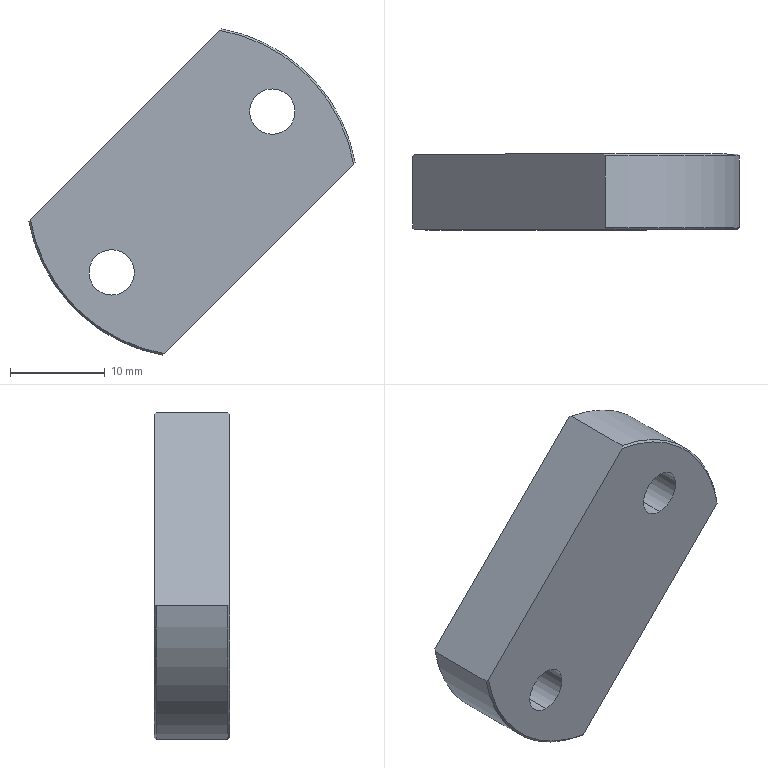Part | SolidWorks | features ICE 3, 3DProfileFeature 2, Chamfer 2, HoleWzd 2, Fillet 1, Revolution 1 | 1 solid | 20 faces | box 34.452 x 8 x 34.452 mm | volume 4691 mm3 | cylinder 10 | plane 6 | cone 4 | commonest cylinder face diameters 4.8 x4 8 x4 35 x2
STEP:
#1=CARTESIAN_POINT('',(-8.485,19.4,-12.485));
#2=VERTEX_POINT('',#1);
#3=CARTESIAN_POINT('',(-8.485,19.4,-4.485));
#4=VERTEX_POINT('',#3);
#5=CARTESIAN_POINT('',(-8.485,19.4,-8.485));
#6=DIRECTION('',(0.,1.,0.));
#7=DIRECTION('',(0.,0.,1.));
#8=AXIS2_PLACEMENT_3D('',#5,#6,#7);
#9=CIRCLE('',#8,4.);
#10=EDGE_CURVE('',#2,#4,#9,.T.);
#11=ORIENTED_EDGE('',*,*,#10,.F.);
#12=CARTESIAN_POINT('',(-8.485,24.,-12.485));
#13=VERTEX_POINT('',#12);
#14=CARTESIAN_POINT('',(-8.485,24.,-12.485));
#15=DIRECTION('',(0.,1.,0.));
#16=VECTOR('',#15,1000.);
#17=LINE('',#14,#16);
#18=EDGE_CURVE('',#2,#13,#17,.T.);
#19=ORIENTED_EDGE('',*,*,#18,.T.);
#20=CARTESIAN_POINT('',(-8.485,24.,-4.485));
#21=VERTEX_POINT('',#20);
#22=CARTESIAN_POINT('',(-8.485,24.,-8.485));
#23=DIRECTION('',(0.,1.,0.));
#24=DIRECTION('',(0.,0.,1.));
#25=AXIS2_PLACEMENT_3D('',#22,#23,#24);
#26=CIRCLE('',#25,4.);
#27=EDGE_CURVE('',#13,#21,#26,.T.);
#28=ORIENTED_EDGE('',*,*,#27,.T.);
#29=CARTESIAN_POINT('',(-8.485,24.,-4.485));
#30=DIRECTION('',(0.,1.,0.));
#31=VECTOR('',#30,1000.);
#32=LINE('',#29,#31);
#33=EDGE_CURVE('',#4,#21,#32,.T.);
#34=ORIENTED_EDGE('',*,*,#33,.F.);
#35=EDGE_LOOP('',(#11,#19,#28,#34));
#36=FACE_OUTER_BOUND('',#35,.T.);
#37=CARTESIAN_POINT('',(-8.485,24.,-8.485));
#38=DIRECTION('',(0.,1.,0.));
#39=DIRECTION('',(0.,0.,1.));
#40=AXIS2_PLACEMENT_3D('',#37,#38,#39);
#41=CYLINDRICAL_SURFACE('',#40,4.);
#42=ADVANCED_FACE('',(#36),#41,.F.);
#43=CARTESIAN_POINT('',(-8.485,16.,-10.885));
#44=VERTEX_POINT('',#43);
#45=CARTESIAN_POINT('',(-8.485,16.,-6.085));
#46=VERTEX_POINT('',#45);
#47=CARTESIAN_POINT('',(-8.485,16.,-8.485));
#48=DIRECTION('',(0.,1.,0.));
#49=DIRECTION('',(0.,0.,1.));
#50=AXIS2_PLACEMENT_3D('',#47,#48,#49);
#51=CIRCLE('',#50,2.4);
#52=EDGE_CURVE('',#44,#46,#51,.T.);
#53=ORIENTED_EDGE('',*,*,#52,.F.);
#54=CARTESIAN_POINT('',(-8.485,19.4,-10.885));
#55=VERTEX_POINT('',#54);
#56=CARTESIAN_POINT('',(-8.485,24.,-10.885));
#57=DIRECTION('',(0.,1.,0.));
#58=VECTOR('',#57,1000.);
#59=LINE('',#56,#58);
#60=EDGE_CURVE('',#44,#55,#59,.T.);
#61=ORIENTED_EDGE('',*,*,#60,.T.);
#62=CARTESIAN_POINT('',(-8.485,19.4,-6.085));
#63=VERTEX_POINT('',#62);
#64=CARTESIAN_POINT('',(-8.485,19.4,-8.485));
#65=DIRECTION('',(0.,1.,0.));
#66=DIRECTION('',(0.,0.,1.));
#67=AXIS2_PLACEMENT_3D('',#64,#65,#66);
#68=CIRCLE('',#67,2.4);
#69=EDGE_CURVE('',#55,#63,#68,.T.);
#70=ORIENTED_EDGE('',*,*,#69,.T.);
#71=CARTESIAN_POINT('',(-8.485,24.,-6.085));
#72=DIRECTION('',(0.,1.,0.));
#73=VECTOR('',#72,1000.);
#74=LINE('',#71,#73);
#75=EDGE_CURVE('',#46,#63,#74,.T.);
#76=ORIENTED_EDGE('',*,*,#75,.F.);
#77=EDGE_LOOP('',(#53,#61,#70,#76));
#78=FACE_OUTER_BOUND('',#77,.T.);
#79=CARTESIAN_POINT('',(-8.485,24.,-8.485));
#80=DIRECTION('',(0.,1.,0.));
#81=DIRECTION('',(0.,0.,1.));
#82=AXIS2_PLACEMENT_3D('',#79,#80,#81);
#83=CYLINDRICAL_SURFACE('',#82,2.4);
#84=ADVANCED_FACE('',(#78),#83,.F.);
#85=CARTESIAN_POINT('',(8.485,19.4,4.485));
#86=VERTEX_POINT('',#85);
#87=CARTESIAN_POINT('',(8.485,19.4,12.485));
#88=VERTEX_POINT('',#87);
#89=CARTESIAN_POINT('',(8.485,19.4,8.485));
#90=DIRECTION('',(0.,1.,0.));
#91=DIRECTION('',(0.,0.,1.));
#92=AXIS2_PLACEMENT_3D('',#89,#90,#91);
#93=CIRCLE('',#92,4.);
#94=EDGE_CURVE('',#86,#88,#93,.T.);
#95=ORIENTED_EDGE('',*,*,#94,.F.);
#96=CARTESIAN_POINT('',(8.485,24.,4.485));
#97=VERTEX_POINT('',#96);
#98=CARTESIAN_POINT('',(8.485,24.,4.485));
#99=DIRECTION('',(0.,1.,0.));
#100=VECTOR('',#99,1000.);
#101=LINE('',#98,#100);
#102=EDGE_CURVE('',#86,#97,#101,.T.);
#103=ORIENTED_EDGE('',*,*,#102,.T.);
#104=CARTESIAN_POINT('',(8.485,24.,12.485));
#105=VERTEX_POINT('',#104);
#106=CARTESIAN_POINT('',(8.485,24.,8.485));
#107=DIRECTION('',(0.,1.,0.));
#108=DIRECTION('',(0.,0.,1.));
#109=AXIS2_PLACEMENT_3D('',#106,#107,#108);
#110=CIRCLE('',#109,4.);
#111=EDGE_CURVE('',#97,#105,#110,.T.);
#112=ORIENTED_EDGE('',*,*,#111,.T.);
#113=CARTESIAN_POINT('',(8.485,24.,12.485));
#114=DIRECTION('',(0.,1.,0.));
#115=VECTOR('',#114,1000.);
#116=LINE('',#113,#115);
#117=EDGE_CURVE('',#88,#105,#116,.T.);
#118=ORIENTED_EDGE('',*,*,#117,.F.);
#119=EDGE_LOOP('',(#95,#103,#112,#118));
#120=FACE_OUTER_BOUND('',#119,.T.);
#121=CARTESIAN_POINT('',(8.485,24.,8.485));
#122=DIRECTION('',(0.,1.,0.));
#123=DIRECTION('',(0.,0.,1.));
#124=AXIS2_PLACEMENT_3D('',#121,#122,#123);
#125=CYLINDRICAL_SURFACE('',#124,4.);
#126=ADVANCED_FACE('',(#120),#125,.F.);
#127=CARTESIAN_POINT('',(8.485,16.,6.085));
#128=VERTEX_POINT('',#127);
#129=CARTESIAN_POINT('',(8.485,16.,10.885));
#130=VERTEX_POINT('',#129);
#131=CARTESIAN_POINT('',(8.485,16.,8.485));
#132=DIRECTION('',(0.,1.,0.));
#133=DIRECTION('',(0.,0.,1.));
#134=AXIS2_PLACEMENT_3D('',#131,#132,#133);
#135=CIRCLE('',#134,2.4);
#136=EDGE_CURVE('',#128,#130,#135,.T.);
#137=ORIENTED_EDGE('',*,*,#136,.F.);
#138=CARTESIAN_POINT('',(8.485,19.4,6.085));
#139=VERTEX_POINT('',#138);
#140=CARTESIAN_POINT('',(8.485,24.,6.085));
#141=DIRECTION('',(0.,1.,0.));
#142=VECTOR('',#141,1000.);
#143=LINE('',#140,#142);
#144=EDGE_CURVE('',#128,#139,#143,.T.);
#145=ORIENTED_EDGE('',*,*,#144,.T.);
#146=CARTESIAN_POINT('',(8.485,19.4,10.885));
#147=VERTEX_POINT('',#146);
#148=CARTESIAN_POINT('',(8.485,19.4,8.485));
#149=DIRECTION('',(0.,1.,0.));
#150=DIRECTION('',(0.,0.,1.));
#151=AXIS2_PLACEMENT_3D('',#148,#149,#150);
#152=CIRCLE('',#151,2.4);
#153=EDGE_CURVE('',#139,#147,#152,.T.);
#154=ORIENTED_EDGE('',*,*,#153,.T.);
#155=CARTESIAN_POINT('',(8.485,24.,10.885));
#156=DIRECTION('',(0.,1.,0.));
#157=VECTOR('',#156,1000.);
#158=LINE('',#155,#157);
#159=EDGE_CURVE('',#130,#147,#158,.T.);
#160=ORIENTED_EDGE('',*,*,#159,.F.);
#161=EDGE_LOOP('',(#137,#145,#154,#160));
#162=FACE_OUTER_BOUND('',#161,.T.);
#163=CARTESIAN_POINT('',(8.485,24.,8.485));
#164=DIRECTION('',(0.,1.,0.));
#165=DIRECTION('',(0.,0.,1.));
#166=AXIS2_PLACEMENT_3D('',#163,#164,#165);
#167=CYLINDRICAL_SURFACE('',#166,2.4);
#168=ADVANCED_FACE('',(#162),#167,.F.);
#169=CARTESIAN_POINT('',(-8.485,24.,-8.485));
#170=DIRECTION('',(0.,1.,0.));
#171=DIRECTION('',(0.,0.,1.));
#172=AXIS2_PLACEMENT_3D('',#169,#170,#171);
#173=CIRCLE('',#172,4.);
#174=EDGE_CURVE('',#21,#13,#173,.T.);
#175=ORIENTED_EDGE('',*,*,#174,.F.);
#176=ORIENTED_EDGE('',*,*,#27,.F.);
#177=EDGE_LOOP('',(#175,#176));
#178=FACE_BOUND('',#177,.T.);
#179=CARTESIAN_POINT('',(8.485,24.,8.485));
#180=DIRECTION('',(0.,1.,0.));
#181=DIRECTION('',(0.,0.,1.));
#182=AXIS2_PLACEMENT_3D('',#179,#180,#181);
#183=CIRCLE('',#182,4.);
#184=EDGE_CURVE('',#105,#97,#183,.T.);
#185=ORIENTED_EDGE('',*,*,#184,.F.);
#186=ORIENTED_EDGE('',*,*,#111,.F.);
#187=EDGE_LOOP('',(#185,#186));
#188=FACE_BOUND('',#187,.T.);
#189=CARTESIAN_POINT('',(2.911,24.,17.053));
#190=VERTEX_POINT('',#189);
#191=CARTESIAN_POINT('',(17.053,24.,2.911));
#192=VERTEX_POINT('',#191);
#193=CARTESIAN_POINT('',(0.,24.,0.));
#194=DIRECTION('',(0.,1.,0.));
#195=DIRECTION('',(0.,0.,-1.));
#196=AXIS2_PLACEMENT_3D('',#193,#194,#195);
#197=CIRCLE('',#196,17.3);
#198=EDGE_CURVE('',#190,#192,#197,.T.);
#199=ORIENTED_EDGE('',*,*,#198,.T.);
#200=CARTESIAN_POINT('',(-2.911,24.,-17.053));
#201=VERTEX_POINT('',#200);
#202=CARTESIAN_POINT('',(7.071,24.,-7.071));
#203=DIRECTION('',(0.7071,0.,0.7071));
#204=VECTOR('',#203,1000.);
#205=LINE('',#202,#204);
#206=EDGE_CURVE('',#201,#192,#205,.T.);
#207=ORIENTED_EDGE('',*,*,#206,.F.);
#208=CARTESIAN_POINT('',(-17.053,24.,-2.911));
#209=VERTEX_POINT('',#208);
#210=CARTESIAN_POINT('',(0.,24.,0.));
#211=DIRECTION('',(0.,1.,0.));
#212=DIRECTION('',(0.,0.,-1.));
#213=AXIS2_PLACEMENT_3D('',#210,#211,#212);
#214=CIRCLE('',#213,17.3);
#215=EDGE_CURVE('',#201,#209,#214,.T.);
#216=ORIENTED_EDGE('',*,*,#215,.T.);
#217=CARTESIAN_POINT('',(-7.071,24.,7.071));
#218=DIRECTION('',(0.7071,0.,0.7071));
#219=VECTOR('',#218,1000.);
#220=LINE('',#217,#219);
#221=EDGE_CURVE('',#209,#190,#220,.T.);
#222=ORIENTED_EDGE('',*,*,#221,.T.);
#223=EDGE_LOOP('',(#199,#207,#216,#222));
#224=FACE_OUTER_BOUND('',#223,.T.);
#225=CARTESIAN_POINT('',(0.,24.,0.));
#226=DIRECTION('',(0.,-1.,0.));
#227=DIRECTION('',(0.,0.,-1.));
#228=AXIS2_PLACEMENT_3D('',#225,#226,#227);
#229=PLANE('',#228);
#230=ADVANCED_FACE('',(#178,#188,#224),#229,.F.);
#231=CARTESIAN_POINT('',(-17.226,23.8,-3.084));
#232=VERTEX_POINT('',#231);
#233=CARTESIAN_POINT('',(-3.084,23.8,-17.226));
#234=VERTEX_POINT('',#233);
#235=CARTESIAN_POINT('',(0.,23.8,0.));
#236=DIRECTION('',(0.,-1.,0.));
#237=DIRECTION('',(0.,0.,-1.));
#238=AXIS2_PLACEMENT_3D('',#235,#236,#237);
#239=CIRCLE('',#238,17.5);
#240=EDGE_CURVE('',#232,#234,#239,.T.);
#241=ORIENTED_EDGE('',*,*,#240,.T.);
#242=CARTESIAN_POINT('',(-3.084,16.2,-17.226));
#243=VERTEX_POINT('',#242);
#244=CARTESIAN_POINT('',(-3.084,0.,-17.226));
#245=DIRECTION('',(0.,1.,0.));
#246=VECTOR('',#245,1000.);
#247=LINE('',#244,#246);
#248=EDGE_CURVE('',#243,#234,#247,.T.);
#249=ORIENTED_EDGE('',*,*,#248,.F.);
#250=CARTESIAN_POINT('',(-17.226,16.2,-3.084));
#251=VERTEX_POINT('',#250);
#252=CARTESIAN_POINT('',(0.,16.2,0.));
#253=DIRECTION('',(0.,1.,0.));
#254=DIRECTION('',(0.,0.,1.));
#255=AXIS2_PLACEMENT_3D('',#252,#253,#254);
#256=CIRCLE('',#255,17.5);
#257=EDGE_CURVE('',#243,#251,#256,.T.);
#258=ORIENTED_EDGE('',*,*,#257,.T.);
#259=CARTESIAN_POINT('',(-17.226,0.,-3.084));
#260=DIRECTION('',(0.,1.,0.));
#261=VECTOR('',#260,1000.);
#262=LINE('',#259,#261);
#263=EDGE_CURVE('',#251,#232,#262,.T.);
#264=ORIENTED_EDGE('',*,*,#263,.T.);
#265=EDGE_LOOP('',(#241,#249,#258,#264));
#266=FACE_OUTER_BOUND('',#265,.T.);
#267=CARTESIAN_POINT('',(0.,0.,0.));
#268=DIRECTION('',(0.,-1.,0.));
#269=DIRECTION('',(0.,0.,-1.));
#270=AXIS2_PLACEMENT_3D('',#267,#268,#269);
#271=CYLINDRICAL_SURFACE('',#270,17.5);
#272=ADVANCED_FACE('',(#266),#271,.T.);
#273=CARTESIAN_POINT('',(3.084,16.2,17.226));
#274=VERTEX_POINT('',#273);
#275=CARTESIAN_POINT('',(17.226,16.2,3.084));
#276=VERTEX_POINT('',#275);
#277=CARTESIAN_POINT('',(0.,16.2,0.));
#278=DIRECTION('',(0.,1.,0.));
#279=DIRECTION('',(0.,0.,1.));
#280=AXIS2_PLACEMENT_3D('',#277,#278,#279);
#281=CIRCLE('',#280,17.5);
#282=EDGE_CURVE('',#274,#276,#281,.T.);
#283=ORIENTED_EDGE('',*,*,#282,.T.);
#284=CARTESIAN_POINT('',(17.226,23.8,3.084));
#285=VERTEX_POINT('',#284);
#286=CARTESIAN_POINT('',(17.226,0.,3.084));
#287=DIRECTION('',(0.,1.,0.));
#288=VECTOR('',#287,1000.);
#289=LINE('',#286,#288);
#290=EDGE_CURVE('',#276,#285,#289,.T.);
#291=ORIENTED_EDGE('',*,*,#290,.T.);
#292=CARTESIAN_POINT('',(3.084,23.8,17.226));
#293=VERTEX_POINT('',#292);
#294=CARTESIAN_POINT('',(0.,23.8,0.));
#295=DIRECTION('',(0.,-1.,0.));
#296=DIRECTION('',(0.,0.,-1.));
#297=AXIS2_PLACEMENT_3D('',#294,#295,#296);
#298=CIRCLE('',#297,17.5);
#299=EDGE_CURVE('',#285,#293,#298,.T.);
#300=ORIENTED_EDGE('',*,*,#299,.T.);
#301=CARTESIAN_POINT('',(3.084,0.,17.226));
#302=DIRECTION('',(0.,1.,0.));
#303=VECTOR('',#302,1000.);
#304=LINE('',#301,#303);
#305=EDGE_CURVE('',#274,#293,#304,.T.);
#306=ORIENTED_EDGE('',*,*,#305,.F.);
#307=EDGE_LOOP('',(#283,#291,#300,#306));
#308=FACE_OUTER_BOUND('',#307,.T.);
#309=CARTESIAN_POINT('',(0.,0.,0.));
#310=DIRECTION('',(0.,-1.,0.));
#311=DIRECTION('',(0.,0.,-1.));
#312=AXIS2_PLACEMENT_3D('',#309,#310,#311);
#313=CYLINDRICAL_SURFACE('',#312,17.5);
#314=ADVANCED_FACE('',(#308),#313,.T.);
#315=CARTESIAN_POINT('',(17.053,16.,2.911));
#316=VERTEX_POINT('',#315);
#317=CARTESIAN_POINT('',(2.911,16.,17.053));
#318=VERTEX_POINT('',#317);
#319=CARTESIAN_POINT('',(0.,16.,0.));
#320=DIRECTION('',(0.,-1.,0.));
#321=DIRECTION('',(0.,0.,1.));
#322=AXIS2_PLACEMENT_3D('',#319,#320,#321);
#323=CIRCLE('',#322,17.3);
#324=EDGE_CURVE('',#316,#318,#323,.T.);
#325=ORIENTED_EDGE('',*,*,#324,.T.);
#326=CARTESIAN_POINT('',(-17.053,16.,-2.911));
#327=VERTEX_POINT('',#326);
#328=CARTESIAN_POINT('',(-15.821,16.,-1.679));
#329=DIRECTION('',(0.7071,0.,0.7071));
#330=VECTOR('',#329,1000.);
#331=LINE('',#328,#330);
#332=EDGE_CURVE('',#327,#318,#331,.T.);
#333=ORIENTED_EDGE('',*,*,#332,.F.);
#334=CARTESIAN_POINT('',(-2.911,16.,-17.053));
#335=VERTEX_POINT('',#334);
#336=CARTESIAN_POINT('',(0.,16.,0.));
#337=DIRECTION('',(0.,-1.,0.));
#338=DIRECTION('',(0.,0.,1.));
#339=AXIS2_PLACEMENT_3D('',#336,#337,#338);
#340=CIRCLE('',#339,17.3);
#341=EDGE_CURVE('',#327,#335,#340,.T.);
#342=ORIENTED_EDGE('',*,*,#341,.T.);
#343=CARTESIAN_POINT('',(-1.679,16.,-15.821));
#344=DIRECTION('',(0.7071,0.,0.7071));
#345=VECTOR('',#344,1000.);
#346=LINE('',#343,#345);
#347=EDGE_CURVE('',#335,#316,#346,.T.);
#348=ORIENTED_EDGE('',*,*,#347,.T.);
#349=EDGE_LOOP('',(#325,#333,#342,#348));
#350=FACE_OUTER_BOUND('',#349,.T.);
#351=CARTESIAN_POINT('',(8.485,16.,8.485));
#352=DIRECTION('',(0.,1.,0.));
#353=DIRECTION('',(0.,0.,1.));
#354=AXIS2_PLACEMENT_3D('',#351,#352,#353);
#355=CIRCLE('',#354,2.4);
#356=EDGE_CURVE('',#130,#128,#355,.T.);
#357=ORIENTED_EDGE('',*,*,#356,.T.);
#358=ORIENTED_EDGE('',*,*,#136,.T.);
#359=EDGE_LOOP('',(#357,#358));
#360=FACE_BOUND('',#359,.T.);
#361=CARTESIAN_POINT('',(-8.485,16.,-8.485));
#362=DIRECTION('',(0.,1.,0.));
#363=DIRECTION('',(0.,0.,1.));
#364=AXIS2_PLACEMENT_3D('',#361,#362,#363);
#365=CIRCLE('',#364,2.4);
#366=EDGE_CURVE('',#46,#44,#365,.T.);
#367=ORIENTED_EDGE('',*,*,#366,.T.);
#368=ORIENTED_EDGE('',*,*,#52,.T.);
#369=EDGE_LOOP('',(#367,#368));
#370=FACE_BOUND('',#369,.T.);
#371=CARTESIAN_POINT('',(-17.5,16.,0.));
#372=DIRECTION('',(0.,1.,0.));
#373=DIRECTION('',(0.,0.,1.));
#374=AXIS2_PLACEMENT_3D('',#371,#372,#373);
#375=PLANE('',#374);
#376=ADVANCED_FACE('',(#350,#360,#370),#375,.F.);
#377=CARTESIAN_POINT('',(-3.084,23.8,-17.226));
#378=CARTESIAN_POINT('',(-3.026,23.867,-17.169));
#379=CARTESIAN_POINT('',(-2.969,23.933,-17.111));
#380=CARTESIAN_POINT('',(-2.911,24.,-17.053));
#381=B_SPLINE_CURVE_WITH_KNOTS('',3,(#377,#378,#379,#380),.UNSPECIFIED.,.F.,.F.,(4,4),(0.02558,0.0259),.UNSPECIFIED.);
#382=EDGE_CURVE('',#234,#201,#381,.T.);
#383=ORIENTED_EDGE('',*,*,#382,.F.);
#384=ORIENTED_EDGE('',*,*,#240,.F.);
#385=CARTESIAN_POINT('',(-17.226,23.8,-3.084));
#386=CARTESIAN_POINT('',(-17.169,23.867,-3.026));
#387=CARTESIAN_POINT('',(-17.111,23.933,-2.969));
#388=CARTESIAN_POINT('',(-17.053,24.,-2.911));
#389=B_SPLINE_CURVE_WITH_KNOTS('',3,(#385,#386,#387,#388),.UNSPECIFIED.,.F.,.F.,(4,4),(0.02558,0.0259),.UNSPECIFIED.);
#390=EDGE_CURVE('',#232,#209,#389,.T.);
#391=ORIENTED_EDGE('',*,*,#390,.T.);
#392=ORIENTED_EDGE('',*,*,#215,.F.);
#393=EDGE_LOOP('',(#383,#384,#391,#392));
#394=FACE_OUTER_BOUND('',#393,.T.);
#395=CARTESIAN_POINT('',(0.,23.8,0.));
#396=DIRECTION('',(0.,-1.,0.));
#397=DIRECTION('',(0.,0.,-1.));
#398=AXIS2_PLACEMENT_3D('',#395,#396,#397);
#399=CONICAL_SURFACE('',#398,17.5,0.7854);
#400=ADVANCED_FACE('',(#394),#399,.T.);
#401=CARTESIAN_POINT('',(17.053,24.,2.911));
#402=CARTESIAN_POINT('',(17.111,23.933,2.969));
#403=CARTESIAN_POINT('',(17.169,23.867,3.026));
#404=CARTESIAN_POINT('',(17.226,23.8,3.084));
#405=B_SPLINE_CURVE_WITH_KNOTS('',3,(#401,#402,#403,#404),.UNSPECIFIED.,.F.,.F.,(4,4),(0.05834,0.05866),.UNSPECIFIED.);
#406=EDGE_CURVE('',#192,#285,#405,.T.);
#407=ORIENTED_EDGE('',*,*,#406,.F.);
#408=ORIENTED_EDGE('',*,*,#198,.F.);
#409=CARTESIAN_POINT('',(2.911,24.,17.053));
#410=CARTESIAN_POINT('',(2.969,23.933,17.111));
#411=CARTESIAN_POINT('',(3.026,23.867,17.169));
#412=CARTESIAN_POINT('',(3.084,23.8,17.226));
#413=B_SPLINE_CURVE_WITH_KNOTS('',3,(#409,#410,#411,#412),.UNSPECIFIED.,.F.,.F.,(4,4),(0.05834,0.05866),.UNSPECIFIED.);
#414=EDGE_CURVE('',#190,#293,#413,.T.);
#415=ORIENTED_EDGE('',*,*,#414,.T.);
#416=ORIENTED_EDGE('',*,*,#299,.F.);
#417=EDGE_LOOP('',(#407,#408,#415,#416));
#418=FACE_OUTER_BOUND('',#417,.T.);
#419=CARTESIAN_POINT('',(0.,23.8,0.));
#420=DIRECTION('',(0.,-1.,0.));
#421=DIRECTION('',(0.,0.,-1.));
#422=AXIS2_PLACEMENT_3D('',#419,#420,#421);
#423=CONICAL_SURFACE('',#422,17.5,0.7854);
#424=ADVANCED_FACE('',(#418),#423,.T.);
#425=CARTESIAN_POINT('',(17.226,16.2,3.084));
#426=CARTESIAN_POINT('',(17.169,16.133,3.026));
#427=CARTESIAN_POINT('',(17.111,16.067,2.969));
#428=CARTESIAN_POINT('',(17.053,16.,2.911));
#429=B_SPLINE_CURVE_WITH_KNOTS('',3,(#425,#426,#427,#428),.UNSPECIFIED.,.F.,.F.,(4,4),(0.02558,0.0259),.UNSPECIFIED.);
#430=EDGE_CURVE('',#276,#316,#429,.T.);
#431=ORIENTED_EDGE('',*,*,#430,.F.);
#432=ORIENTED_EDGE('',*,*,#282,.F.);
#433=CARTESIAN_POINT('',(3.084,16.2,17.226));
#434=CARTESIAN_POINT('',(3.026,16.133,17.169));
#435=CARTESIAN_POINT('',(2.969,16.067,17.111));
#436=CARTESIAN_POINT('',(2.911,16.,17.053));
#437=B_SPLINE_CURVE_WITH_KNOTS('',3,(#433,#434,#435,#436),.UNSPECIFIED.,.F.,.F.,(4,4),(0.02558,0.0259),.UNSPECIFIED.);
#438=EDGE_CURVE('',#274,#318,#437,.T.);
#439=ORIENTED_EDGE('',*,*,#438,.T.);
#440=ORIENTED_EDGE('',*,*,#324,.F.);
#441=EDGE_LOOP('',(#431,#432,#439,#440));
#442=FACE_OUTER_BOUND('',#441,.T.);
#443=CARTESIAN_POINT('',(0.,16.,0.));
#444=DIRECTION('',(0.,1.,0.));
#445=DIRECTION('',(0.,0.,1.));
#446=AXIS2_PLACEMENT_3D('',#443,#444,#445);
#447=CONICAL_SURFACE('',#446,17.3,0.7854);
#448=ADVANCED_FACE('',(#442),#447,.T.);
#449=CARTESIAN_POINT('',(-2.911,16.,-17.053));
#450=CARTESIAN_POINT('',(-2.969,16.067,-17.111));
#451=CARTESIAN_POINT('',(-3.026,16.133,-17.169));
#452=CARTESIAN_POINT('',(-3.084,16.2,-17.226));
#453=B_SPLINE_CURVE_WITH_KNOTS('',3,(#449,#450,#451,#452),.UNSPECIFIED.,.F.,.F.,(4,4),(0.05834,0.05866),.UNSPECIFIED.);
#454=EDGE_CURVE('',#335,#243,#453,.T.);
#455=ORIENTED_EDGE('',*,*,#454,.F.);
#456=ORIENTED_EDGE('',*,*,#341,.F.);
#457=CARTESIAN_POINT('',(-17.053,16.,-2.911));
#458=CARTESIAN_POINT('',(-17.111,16.067,-2.969));
#459=CARTESIAN_POINT('',(-17.169,16.133,-3.026));
#460=CARTESIAN_POINT('',(-17.226,16.2,-3.084));
#461=B_SPLINE_CURVE_WITH_KNOTS('',3,(#457,#458,#459,#460),.UNSPECIFIED.,.F.,.F.,(4,4),(0.05834,0.05866),.UNSPECIFIED.);
#462=EDGE_CURVE('',#327,#251,#461,.T.);
#463=ORIENTED_EDGE('',*,*,#462,.T.);
#464=ORIENTED_EDGE('',*,*,#257,.F.);
#465=EDGE_LOOP('',(#455,#456,#463,#464));
#466=FACE_OUTER_BOUND('',#465,.T.);
#467=CARTESIAN_POINT('',(0.,16.,0.));
#468=DIRECTION('',(0.,1.,0.));
#469=DIRECTION('',(0.,0.,1.));
#470=AXIS2_PLACEMENT_3D('',#467,#468,#469);
#471=CONICAL_SURFACE('',#470,17.3,0.7854);
#472=ADVANCED_FACE('',(#466),#471,.T.);
#473=ORIENTED_EDGE('',*,*,#144,.F.);
#474=ORIENTED_EDGE('',*,*,#356,.F.);
#475=ORIENTED_EDGE('',*,*,#159,.T.);
#476=CARTESIAN_POINT('',(8.485,19.4,8.485));
#477=DIRECTION('',(0.,1.,0.));
#478=DIRECTION('',(0.,0.,1.));
#479=AXIS2_PLACEMENT_3D('',#476,#477,#478);
#480=CIRCLE('',#479,2.4);
#481=EDGE_CURVE('',#147,#139,#480,.T.);
#482=ORIENTED_EDGE('',*,*,#481,.T.);
#483=EDGE_LOOP('',(#473,#474,#475,#482));
#484=FACE_OUTER_BOUND('',#483,.T.);
#485=CARTESIAN_POINT('',(8.485,24.,8.485));
#486=DIRECTION('',(0.,1.,0.));
#487=DIRECTION('',(0.,0.,1.));
#488=AXIS2_PLACEMENT_3D('',#485,#486,#487);
#489=CYLINDRICAL_SURFACE('',#488,2.4);
#490=ADVANCED_FACE('',(#484),#489,.F.);
#491=ORIENTED_EDGE('',*,*,#481,.F.);
#492=ORIENTED_EDGE('',*,*,#153,.F.);
#493=EDGE_LOOP('',(#491,#492));
#494=FACE_BOUND('',#493,.T.);
#495=CARTESIAN_POINT('',(8.485,19.4,8.485));
#496=DIRECTION('',(0.,1.,0.));
#497=DIRECTION('',(0.,0.,1.));
#498=AXIS2_PLACEMENT_3D('',#495,#496,#497);
#499=CIRCLE('',#498,4.);
#500=EDGE_CURVE('',#88,#86,#499,.T.);
#501=ORIENTED_EDGE('',*,*,#500,.T.);
#502=ORIENTED_EDGE('',*,*,#94,.T.);
#503=EDGE_LOOP('',(#501,#502));
#504=FACE_OUTER_BOUND('',#503,.T.);
#505=CARTESIAN_POINT('',(10.885,19.4,8.485));
#506=DIRECTION('',(0.,-1.,0.));
#507=DIRECTION('',(0.,0.,-1.));
#508=AXIS2_PLACEMENT_3D('',#505,#506,#507);
#509=PLANE('',#508);
#510=ADVANCED_FACE('',(#494,#504),#509,.F.);
#511=ORIENTED_EDGE('',*,*,#102,.F.);
#512=ORIENTED_EDGE('',*,*,#500,.F.);
#513=ORIENTED_EDGE('',*,*,#117,.T.);
#514=ORIENTED_EDGE('',*,*,#184,.T.);
#515=EDGE_LOOP('',(#511,#512,#513,#514));
#516=FACE_OUTER_BOUND('',#515,.T.);
#517=CARTESIAN_POINT('',(8.485,24.,8.485));
#518=DIRECTION('',(0.,1.,0.));
#519=DIRECTION('',(0.,0.,1.));
#520=AXIS2_PLACEMENT_3D('',#517,#518,#519);
#521=CYLINDRICAL_SURFACE('',#520,4.);
#522=ADVANCED_FACE('',(#516),#521,.F.);
#523=ORIENTED_EDGE('',*,*,#60,.F.);
#524=ORIENTED_EDGE('',*,*,#366,.F.);
#525=ORIENTED_EDGE('',*,*,#75,.T.);
#526=CARTESIAN_POINT('',(-8.485,19.4,-8.485));
#527=DIRECTION('',(0.,1.,0.));
#528=DIRECTION('',(0.,0.,1.));
#529=AXIS2_PLACEMENT_3D('',#526,#527,#528);
#530=CIRCLE('',#529,2.4);
#531=EDGE_CURVE('',#63,#55,#530,.T.);
#532=ORIENTED_EDGE('',*,*,#531,.T.);
#533=EDGE_LOOP('',(#523,#524,#525,#532));
#534=FACE_OUTER_BOUND('',#533,.T.);
#535=CARTESIAN_POINT('',(-8.485,24.,-8.485));
#536=DIRECTION('',(0.,1.,0.));
#537=DIRECTION('',(0.,0.,1.));
#538=AXIS2_PLACEMENT_3D('',#535,#536,#537);
#539=CYLINDRICAL_SURFACE('',#538,2.4);
#540=ADVANCED_FACE('',(#534),#539,.F.);
#541=ORIENTED_EDGE('',*,*,#531,.F.);
#542=ORIENTED_EDGE('',*,*,#69,.F.);
#543=EDGE_LOOP('',(#541,#542));
#544=FACE_BOUND('',#543,.T.);
#545=CARTESIAN_POINT('',(-8.485,19.4,-8.485));
#546=DIRECTION('',(0.,1.,0.));
#547=DIRECTION('',(0.,0.,1.));
#548=AXIS2_PLACEMENT_3D('',#545,#546,#547);
#549=CIRCLE('',#548,4.);
#550=EDGE_CURVE('',#4,#2,#549,.T.);
#551=ORIENTED_EDGE('',*,*,#550,.T.);
#552=ORIENTED_EDGE('',*,*,#10,.T.);
#553=EDGE_LOOP('',(#551,#552));
#554=FACE_OUTER_BOUND('',#553,.T.);
#555=CARTESIAN_POINT('',(-6.085,19.4,-8.485));
#556=DIRECTION('',(0.,-1.,0.));
#557=DIRECTION('',(0.,0.,-1.));
#558=AXIS2_PLACEMENT_3D('',#555,#556,#557);
#559=PLANE('',#558);
#560=ADVANCED_FACE('',(#544,#554),#559,.F.);
#561=ORIENTED_EDGE('',*,*,#18,.F.);
#562=ORIENTED_EDGE('',*,*,#550,.F.);
#563=ORIENTED_EDGE('',*,*,#33,.T.);
#564=ORIENTED_EDGE('',*,*,#174,.T.);
#565=EDGE_LOOP('',(#561,#562,#563,#564));
#566=FACE_OUTER_BOUND('',#565,.T.);
#567=CARTESIAN_POINT('',(-8.485,24.,-8.485));
#568=DIRECTION('',(0.,1.,0.));
#569=DIRECTION('',(0.,0.,1.));
#570=AXIS2_PLACEMENT_3D('',#567,#568,#569);
#571=CYLINDRICAL_SURFACE('',#570,4.);
#572=ADVANCED_FACE('',(#566),#571,.F.);
#573=ORIENTED_EDGE('',*,*,#263,.F.);
#574=ORIENTED_EDGE('',*,*,#462,.F.);
#575=ORIENTED_EDGE('',*,*,#332,.T.);
#576=ORIENTED_EDGE('',*,*,#438,.F.);
#577=ORIENTED_EDGE('',*,*,#305,.T.);
#578=ORIENTED_EDGE('',*,*,#414,.F.);
#579=ORIENTED_EDGE('',*,*,#221,.F.);
#580=ORIENTED_EDGE('',*,*,#390,.F.);
#581=EDGE_LOOP('',(#573,#574,#575,#576,#577,#578,#579,#580));
#582=FACE_OUTER_BOUND('',#581,.T.);
#583=CARTESIAN_POINT('',(-7.071,0.,7.071));
#584=DIRECTION('',(-0.7071,0.,0.7071));
#585=DIRECTION('',(0.7071,0.,0.7071));
#586=AXIS2_PLACEMENT_3D('',#583,#584,#585);
#587=PLANE('',#586);
#588=ADVANCED_FACE('',(#582),#587,.T.);
#589=ORIENTED_EDGE('',*,*,#382,.T.);
#590=ORIENTED_EDGE('',*,*,#206,.T.);
#591=ORIENTED_EDGE('',*,*,#406,.T.);
#592=ORIENTED_EDGE('',*,*,#290,.F.);
#593=ORIENTED_EDGE('',*,*,#430,.T.);
#594=ORIENTED_EDGE('',*,*,#347,.F.);
#595=ORIENTED_EDGE('',*,*,#454,.T.);
#596=ORIENTED_EDGE('',*,*,#248,.T.);
#597=EDGE_LOOP('',(#589,#590,#591,#592,#593,#594,#595,#596));
#598=FACE_OUTER_BOUND('',#597,.T.);
#599=CARTESIAN_POINT('',(7.071,0.,-7.071));
#600=DIRECTION('',(-0.7071,0.,0.7071));
#601=DIRECTION('',(0.7071,0.,0.7071));
#602=AXIS2_PLACEMENT_3D('',#599,#600,#601);
#603=PLANE('',#602);
#604=ADVANCED_FACE('',(#598),#603,.F.);
#605=CLOSED_SHELL('',(#42,#84,#126,#168,#230,#272,#314,#376,#400,#424,#448,#472,#490,#510,#522,#540,#560,#572,#588,#604));
#606=MANIFOLD_SOLID_BREP('',#605);
#607=CARTESIAN_POINT('',(0.,0.,0.));
#608=DIRECTION('',(0.,0.,1.));
#609=DIRECTION('',(1.,0.,0.));
#610=AXIS2_PLACEMENT_3D('',#607,#608,#609);
#611=(LENGTH_UNIT()NAMED_UNIT(*)SI_UNIT(.MILLI.,.METRE.));
#612=UNCERTAINTY_MEASURE_WITH_UNIT(LENGTH_MEASURE(0.00001),#611,'','');
#613=(NAMED_UNIT(*)PLANE_ANGLE_UNIT()SI_UNIT($,.RADIAN.));
#614=(NAMED_UNIT(*)SI_UNIT($,.STERADIAN.)SOLID_ANGLE_UNIT());
#615=(GEOMETRIC_REPRESENTATION_CONTEXT(3)GLOBAL_UNCERTAINTY_ASSIGNED_CONTEXT((#612))GLOBAL_UNIT_ASSIGNED_CONTEXT((#611,#613,#614))REPRESENTATION_CONTEXT('',''));
#616=ADVANCED_BREP_SHAPE_REPRESENTATION('',(#606,#610),#615);